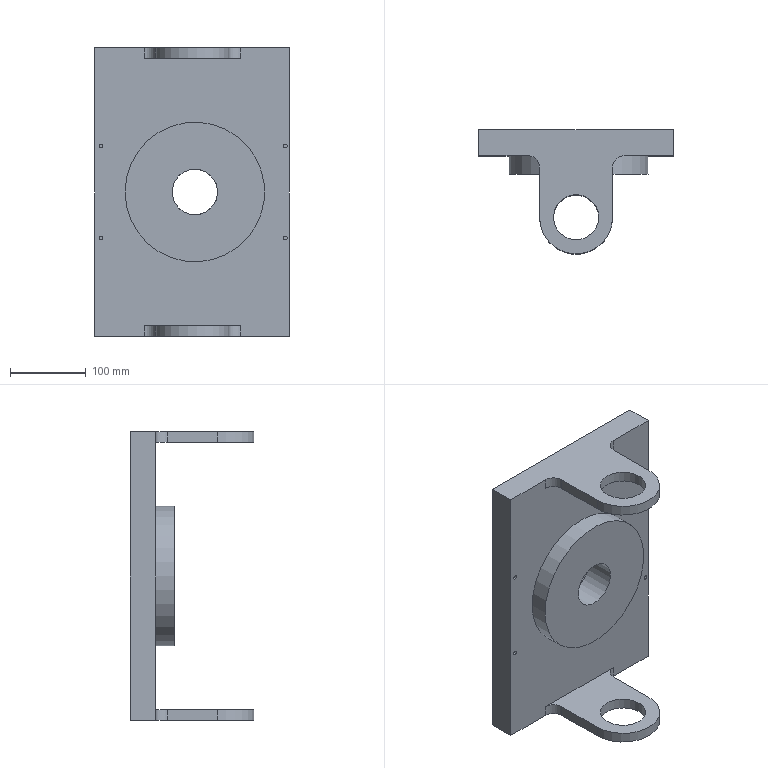Part | NX | features BREP 3 | 3 solids | 41 faces | box 256 x 163.215 x 380 mm | volume 4024571 mm3 | plane 22 | cylinder 19 | commonest cylinder face diameters 5 x4 30 x4 59.433 x2 60 x2 95 x2 96.269 x2
STEP:
#1=CARTESIAN_POINT('',(18.91,256.,-98.298));
#2=VERTEX_POINT('',#1);
#3=CARTESIAN_POINT('',(21.41,256.,-98.298));
#4=DIRECTION('',(0.,1.,0.));
#5=DIRECTION('',(-1.,0.,0.));
#6=AXIS2_PLACEMENT_3D('',#3,#4,#5);
#7=CIRCLE('',#6,2.5);
#8=EDGE_CURVE('',#2,#2,#7,.T.);
#9=ORIENTED_EDGE('',*,*,#8,.T.);
#10=EDGE_LOOP('',(#9));
#11=FACE_BOUND('',#10,.T.);
#12=CARTESIAN_POINT('',(-223.757,256.,-219.702));
#13=VERTEX_POINT('',#12);
#14=CARTESIAN_POINT('',(-221.257,256.,-219.702));
#15=DIRECTION('',(0.,1.,0.));
#16=DIRECTION('',(-1.,0.,0.));
#17=AXIS2_PLACEMENT_3D('',#14,#15,#16);
#18=CIRCLE('',#17,2.5);
#19=EDGE_CURVE('',#13,#13,#18,.T.);
#20=ORIENTED_EDGE('',*,*,#19,.T.);
#21=EDGE_LOOP('',(#20));
#22=FACE_BOUND('',#21,.T.);
#23=CARTESIAN_POINT('',(-189.579,256.,-159.));
#24=VERTEX_POINT('',#23);
#25=CARTESIAN_POINT('',(-97.711,256.,-159.));
#26=DIRECTION('',(0.,-1.,0.));
#27=DIRECTION('',(-1.,0.,0.));
#28=AXIS2_PLACEMENT_3D('',#25,#26,#27);
#29=CIRCLE('',#28,91.868);
#30=EDGE_CURVE('',#24,#24,#29,.T.);
#31=ORIENTED_EDGE('',*,*,#30,.F.);
#32=EDGE_LOOP('',(#31));
#33=FACE_BOUND('',#32,.T.);
#34=CARTESIAN_POINT('',(-38.221,256.,31.));
#35=VERTEX_POINT('',#34);
#36=CARTESIAN_POINT('',(26.51,256.,31.));
#37=VERTEX_POINT('',#36);
#38=CARTESIAN_POINT('',(26.51,256.,31.));
#39=DIRECTION('',(1.,0.,0.));
#40=VECTOR('',#39,1000.);
#41=LINE('',#38,#40);
#42=EDGE_CURVE('',#35,#37,#41,.T.);
#43=ORIENTED_EDGE('',*,*,#42,.F.);
#44=CARTESIAN_POINT('',(-38.221,256.,17.));
#45=VERTEX_POINT('',#44);
#46=CARTESIAN_POINT('',(-38.221,256.,17.));
#47=DIRECTION('',(0.,0.,-1.));
#48=VECTOR('',#47,1000.);
#49=LINE('',#46,#48);
#50=EDGE_CURVE('',#35,#45,#49,.T.);
#51=ORIENTED_EDGE('',*,*,#50,.T.);
#52=CARTESIAN_POINT('',(-164.49,256.,17.));
#53=VERTEX_POINT('',#52);
#54=CARTESIAN_POINT('',(-1006.286,256.,17.));
#55=DIRECTION('',(1.,0.,0.));
#56=VECTOR('',#55,1000.);
#57=LINE('',#54,#56);
#58=EDGE_CURVE('',#53,#45,#57,.T.);
#59=ORIENTED_EDGE('',*,*,#58,.F.);
#60=CARTESIAN_POINT('',(-164.49,256.,31.));
#61=VERTEX_POINT('',#60);
#62=CARTESIAN_POINT('',(-164.49,256.,31.));
#63=DIRECTION('',(0.,0.,1.));
#64=VECTOR('',#63,1000.);
#65=LINE('',#62,#64);
#66=EDGE_CURVE('',#53,#61,#65,.T.);
#67=ORIENTED_EDGE('',*,*,#66,.T.);
#68=CARTESIAN_POINT('',(-229.49,256.,31.));
#69=VERTEX_POINT('',#68);
#70=CARTESIAN_POINT('',(-229.49,256.,31.));
#71=DIRECTION('',(1.,0.,0.));
#72=VECTOR('',#71,1000.);
#73=LINE('',#70,#72);
#74=EDGE_CURVE('',#69,#61,#73,.T.);
#75=ORIENTED_EDGE('',*,*,#74,.F.);
#76=CARTESIAN_POINT('',(-229.49,256.,-349.));
#77=VERTEX_POINT('',#76);
#78=CARTESIAN_POINT('',(-229.49,256.,-349.));
#79=DIRECTION('',(0.,0.,1.));
#80=VECTOR('',#79,1000.);
#81=LINE('',#78,#80);
#82=EDGE_CURVE('',#77,#69,#81,.T.);
#83=ORIENTED_EDGE('',*,*,#82,.F.);
#84=CARTESIAN_POINT('',(-164.49,256.,-349.));
#85=VERTEX_POINT('',#84);
#86=CARTESIAN_POINT('',(-229.49,256.,-349.));
#87=DIRECTION('',(-1.,0.,0.));
#88=VECTOR('',#87,1000.);
#89=LINE('',#86,#88);
#90=EDGE_CURVE('',#85,#77,#89,.T.);
#91=ORIENTED_EDGE('',*,*,#90,.F.);
#92=CARTESIAN_POINT('',(-164.49,256.,-335.));
#93=VERTEX_POINT('',#92);
#94=CARTESIAN_POINT('',(-164.49,256.,-335.));
#95=DIRECTION('',(0.,0.,1.));
#96=VECTOR('',#95,1000.);
#97=LINE('',#94,#96);
#98=EDGE_CURVE('',#85,#93,#97,.T.);
#99=ORIENTED_EDGE('',*,*,#98,.T.);
#100=CARTESIAN_POINT('',(-38.221,256.,-335.));
#101=VERTEX_POINT('',#100);
#102=CARTESIAN_POINT('',(-1006.286,256.,-335.));
#103=DIRECTION('',(-1.,0.,0.));
#104=VECTOR('',#103,1000.);
#105=LINE('',#102,#104);
#106=EDGE_CURVE('',#101,#93,#105,.T.);
#107=ORIENTED_EDGE('',*,*,#106,.F.);
#108=CARTESIAN_POINT('',(-38.221,256.,-349.));
#109=VERTEX_POINT('',#108);
#110=CARTESIAN_POINT('',(-38.221,256.,-349.));
#111=DIRECTION('',(0.,0.,-1.));
#112=VECTOR('',#111,1000.);
#113=LINE('',#110,#112);
#114=EDGE_CURVE('',#101,#109,#113,.T.);
#115=ORIENTED_EDGE('',*,*,#114,.T.);
#116=CARTESIAN_POINT('',(26.51,256.,-349.));
#117=VERTEX_POINT('',#116);
#118=CARTESIAN_POINT('',(26.51,256.,-349.));
#119=DIRECTION('',(-1.,0.,0.));
#120=VECTOR('',#119,1000.);
#121=LINE('',#118,#120);
#122=EDGE_CURVE('',#117,#109,#121,.T.);
#123=ORIENTED_EDGE('',*,*,#122,.F.);
#124=CARTESIAN_POINT('',(26.51,256.,31.));
#125=DIRECTION('',(0.,0.,-1.));
#126=VECTOR('',#125,1000.);
#127=LINE('',#124,#126);
#128=EDGE_CURVE('',#37,#117,#127,.T.);
#129=ORIENTED_EDGE('',*,*,#128,.F.);
#130=EDGE_LOOP('',(#43,#51,#59,#67,#75,#83,#91,#99,#107,#115,#123,#129));
#131=FACE_BOUND('',#130,.T.);
#132=CARTESIAN_POINT('',(18.91,256.,-219.702));
#133=VERTEX_POINT('',#132);
#134=CARTESIAN_POINT('',(21.41,256.,-219.702));
#135=DIRECTION('',(0.,-1.,0.));
#136=DIRECTION('',(-1.,0.,0.));
#137=AXIS2_PLACEMENT_3D('',#134,#135,#136);
#138=CIRCLE('',#137,2.5);
#139=EDGE_CURVE('',#133,#133,#138,.T.);
#140=ORIENTED_EDGE('',*,*,#139,.F.);
#141=EDGE_LOOP('',(#140));
#142=FACE_BOUND('',#141,.T.);
#143=CARTESIAN_POINT('',(-223.757,256.,-98.298));
#144=VERTEX_POINT('',#143);
#145=CARTESIAN_POINT('',(-221.257,256.,-98.298));
#146=DIRECTION('',(0.,-1.,0.));
#147=DIRECTION('',(-1.,0.,0.));
#148=AXIS2_PLACEMENT_3D('',#145,#146,#147);
#149=CIRCLE('',#148,2.5);
#150=EDGE_CURVE('',#144,#144,#149,.T.);
#151=ORIENTED_EDGE('',*,*,#150,.F.);
#152=EDGE_LOOP('',(#151));
#153=FACE_BOUND('',#152,.T.);
#154=CARTESIAN_POINT('',(26.51,256.,31.));
#155=DIRECTION('',(0.,1.,0.));
#156=DIRECTION('',(1.,0.,0.));
#157=AXIS2_PLACEMENT_3D('',#154,#155,#156);
#158=PLANE('',#157);
#159=ADVANCED_FACE('',(#11,#22,#33,#131,#142,#153),#158,.F.);
#160=CARTESIAN_POINT('',(-97.711,232.,-189.));
#161=VERTEX_POINT('',#160);
#162=CARTESIAN_POINT('',(-97.711,232.,-159.));
#163=DIRECTION('',(0.,-1.,0.));
#164=DIRECTION('',(0.,0.,-1.));
#165=AXIS2_PLACEMENT_3D('',#162,#163,#164);
#166=CIRCLE('',#165,30.);
#167=EDGE_CURVE('',#161,#161,#166,.T.);
#168=ORIENTED_EDGE('',*,*,#167,.T.);
#169=EDGE_LOOP('',(#168));
#170=FACE_BOUND('',#169,.T.);
#171=CARTESIAN_POINT('',(-97.711,272.,-129.));
#172=VERTEX_POINT('',#171);
#173=CARTESIAN_POINT('',(-97.711,272.,-159.));
#174=DIRECTION('',(0.,-1.,0.));
#175=DIRECTION('',(0.,0.,1.));
#176=AXIS2_PLACEMENT_3D('',#173,#174,#175);
#177=CIRCLE('',#176,30.);
#178=EDGE_CURVE('',#172,#172,#177,.T.);
#179=ORIENTED_EDGE('',*,*,#178,.F.);
#180=EDGE_LOOP('',(#179));
#181=FACE_BOUND('',#180,.T.);
#182=CARTESIAN_POINT('',(-97.711,315.,-159.));
#183=DIRECTION('',(0.,-1.,0.));
#184=DIRECTION('',(-1.,0.,0.));
#185=AXIS2_PLACEMENT_3D('',#182,#183,#184);
#186=CYLINDRICAL_SURFACE('',#185,30.);
#187=ADVANCED_FACE('',(#170,#181),#186,.F.);
#188=ORIENTED_EDGE('',*,*,#122,.T.);
#189=CARTESIAN_POINT('',(-53.221,241.,-349.));
#190=VERTEX_POINT('',#189);
#191=CARTESIAN_POINT('',(-38.221,241.,-349.));
#192=DIRECTION('',(0.,0.,1.));
#193=DIRECTION('',(0.,-1.,0.));
#194=AXIS2_PLACEMENT_3D('',#191,#192,#193);
#195=CIRCLE('',#194,15.);
#196=EDGE_CURVE('',#109,#190,#195,.T.);
#197=ORIENTED_EDGE('',*,*,#196,.T.);
#198=CARTESIAN_POINT('',(-53.221,174.92,-349.));
#199=VERTEX_POINT('',#198);
#200=CARTESIAN_POINT('',(-53.221,290.,-349.));
#201=DIRECTION('',(0.,1.,0.));
#202=VECTOR('',#201,1000.);
#203=LINE('',#200,#202);
#204=EDGE_CURVE('',#199,#190,#203,.T.);
#205=ORIENTED_EDGE('',*,*,#204,.F.);
#206=CARTESIAN_POINT('',(-149.49,174.92,-349.));
#207=VERTEX_POINT('',#206);
#208=CARTESIAN_POINT('',(-101.355,174.92,-349.));
#209=DIRECTION('',(0.,0.,1.));
#210=DIRECTION('',(-1.,0.,0.));
#211=AXIS2_PLACEMENT_3D('',#208,#209,#210);
#212=CIRCLE('',#211,48.135);
#213=EDGE_CURVE('',#207,#199,#212,.T.);
#214=ORIENTED_EDGE('',*,*,#213,.F.);
#215=CARTESIAN_POINT('',(-149.49,241.,-349.));
#216=VERTEX_POINT('',#215);
#217=CARTESIAN_POINT('',(-149.49,174.92,-349.));
#218=DIRECTION('',(0.,-1.,0.));
#219=VECTOR('',#218,1000.);
#220=LINE('',#217,#219);
#221=EDGE_CURVE('',#216,#207,#220,.T.);
#222=ORIENTED_EDGE('',*,*,#221,.F.);
#223=CARTESIAN_POINT('',(-164.49,241.,-349.));
#224=DIRECTION('',(0.,0.,1.));
#225=DIRECTION('',(0.,-1.,0.));
#226=AXIS2_PLACEMENT_3D('',#223,#224,#225);
#227=CIRCLE('',#226,15.);
#228=EDGE_CURVE('',#216,#85,#227,.T.);
#229=ORIENTED_EDGE('',*,*,#228,.T.);
#230=ORIENTED_EDGE('',*,*,#90,.T.);
#231=CARTESIAN_POINT('',(-229.49,290.,-349.));
#232=VERTEX_POINT('',#231);
#233=CARTESIAN_POINT('',(-229.49,290.,-349.));
#234=DIRECTION('',(0.,-1.,0.));
#235=VECTOR('',#234,1000.);
#236=LINE('',#233,#235);
#237=EDGE_CURVE('',#232,#77,#236,.T.);
#238=ORIENTED_EDGE('',*,*,#237,.F.);
#239=CARTESIAN_POINT('',(26.51,290.,-349.));
#240=VERTEX_POINT('',#239);
#241=CARTESIAN_POINT('',(26.51,290.,-349.));
#242=DIRECTION('',(-1.,0.,0.));
#243=VECTOR('',#242,1000.);
#244=LINE('',#241,#243);
#245=EDGE_CURVE('',#240,#232,#244,.T.);
#246=ORIENTED_EDGE('',*,*,#245,.F.);
#247=CARTESIAN_POINT('',(26.51,256.,-349.));
#248=DIRECTION('',(0.,1.,0.));
#249=VECTOR('',#248,1000.);
#250=LINE('',#247,#249);
#251=EDGE_CURVE('',#117,#240,#250,.T.);
#252=ORIENTED_EDGE('',*,*,#251,.F.);
#253=EDGE_LOOP('',(#188,#197,#205,#214,#222,#229,#230,#238,#246,#252));
#254=FACE_BOUND('',#253,.T.);
#255=CARTESIAN_POINT('',(-131.072,174.92,-349.));
#256=VERTEX_POINT('',#255);
#257=CARTESIAN_POINT('',(-101.355,174.92,-349.));
#258=DIRECTION('',(0.,0.,1.));
#259=DIRECTION('',(-1.,0.,0.));
#260=AXIS2_PLACEMENT_3D('',#257,#258,#259);
#261=CIRCLE('',#260,29.717);
#262=EDGE_CURVE('',#256,#256,#261,.T.);
#263=ORIENTED_EDGE('',*,*,#262,.T.);
#264=EDGE_LOOP('',(#263));
#265=FACE_BOUND('',#264,.T.);
#266=CARTESIAN_POINT('',(26.51,256.,-349.));
#267=DIRECTION('',(0.,0.,1.));
#268=DIRECTION('',(0.,1.,0.));
#269=AXIS2_PLACEMENT_3D('',#266,#267,#268);
#270=PLANE('',#269);
#271=ADVANCED_FACE('',(#254,#265),#270,.F.);
#272=CARTESIAN_POINT('',(-32.711,290.,-159.));
#273=VERTEX_POINT('',#272);
#274=CARTESIAN_POINT('',(-97.711,290.,-159.));
#275=DIRECTION('',(0.,-1.,0.));
#276=DIRECTION('',(1.,0.,0.));
#277=AXIS2_PLACEMENT_3D('',#274,#275,#276);
#278=CIRCLE('',#277,65.);
#279=EDGE_CURVE('',#273,#273,#278,.T.);
#280=ORIENTED_EDGE('',*,*,#279,.T.);
#281=EDGE_LOOP('',(#280));
#282=FACE_BOUND('',#281,.T.);
#283=ORIENTED_EDGE('',*,*,#245,.T.);
#284=CARTESIAN_POINT('',(-229.49,290.,31.));
#285=VERTEX_POINT('',#284);
#286=CARTESIAN_POINT('',(-229.49,290.,31.));
#287=DIRECTION('',(0.,0.,-1.));
#288=VECTOR('',#287,1000.);
#289=LINE('',#286,#288);
#290=EDGE_CURVE('',#285,#232,#289,.T.);
#291=ORIENTED_EDGE('',*,*,#290,.F.);
#292=CARTESIAN_POINT('',(26.51,290.,31.));
#293=VERTEX_POINT('',#292);
#294=CARTESIAN_POINT('',(26.51,290.,31.));
#295=DIRECTION('',(1.,0.,0.));
#296=VECTOR('',#295,1000.);
#297=LINE('',#294,#296);
#298=EDGE_CURVE('',#285,#293,#297,.T.);
#299=ORIENTED_EDGE('',*,*,#298,.T.);
#300=CARTESIAN_POINT('',(26.51,290.,-349.));
#301=DIRECTION('',(0.,0.,1.));
#302=VECTOR('',#301,1000.);
#303=LINE('',#300,#302);
#304=EDGE_CURVE('',#240,#293,#303,.T.);
#305=ORIENTED_EDGE('',*,*,#304,.F.);
#306=EDGE_LOOP('',(#283,#291,#299,#305));
#307=FACE_BOUND('',#306,.T.);
#308=CARTESIAN_POINT('',(26.51,290.,-349.));
#309=DIRECTION('',(0.,-1.,0.));
#310=DIRECTION('',(-1.,0.,0.));
#311=AXIS2_PLACEMENT_3D('',#308,#309,#310);
#312=PLANE('',#311);
#313=ADVANCED_FACE('',(#282,#307),#312,.F.);
#314=ORIENTED_EDGE('',*,*,#298,.F.);
#315=CARTESIAN_POINT('',(-229.49,256.,31.));
#316=DIRECTION('',(0.,1.,0.));
#317=VECTOR('',#316,1000.);
#318=LINE('',#315,#317);
#319=EDGE_CURVE('',#69,#285,#318,.T.);
#320=ORIENTED_EDGE('',*,*,#319,.F.);
#321=ORIENTED_EDGE('',*,*,#74,.T.);
#322=CARTESIAN_POINT('',(-149.49,241.,31.));
#323=VERTEX_POINT('',#322);
#324=CARTESIAN_POINT('',(-164.49,241.,31.));
#325=DIRECTION('',(0.,0.,-1.));
#326=DIRECTION('',(-1.,0.,0.));
#327=AXIS2_PLACEMENT_3D('',#324,#325,#326);
#328=CIRCLE('',#327,15.);
#329=EDGE_CURVE('',#61,#323,#328,.T.);
#330=ORIENTED_EDGE('',*,*,#329,.T.);
#331=CARTESIAN_POINT('',(-149.49,174.92,31.));
#332=VERTEX_POINT('',#331);
#333=CARTESIAN_POINT('',(-149.49,174.92,31.));
#334=DIRECTION('',(0.,1.,0.));
#335=VECTOR('',#334,1000.);
#336=LINE('',#333,#335);
#337=EDGE_CURVE('',#332,#323,#336,.T.);
#338=ORIENTED_EDGE('',*,*,#337,.F.);
#339=CARTESIAN_POINT('',(-53.221,174.92,31.));
#340=VERTEX_POINT('',#339);
#341=CARTESIAN_POINT('',(-101.355,174.92,31.));
#342=DIRECTION('',(0.,0.,-1.));
#343=DIRECTION('',(-1.,0.,0.));
#344=AXIS2_PLACEMENT_3D('',#341,#342,#343);
#345=CIRCLE('',#344,48.135);
#346=EDGE_CURVE('',#340,#332,#345,.T.);
#347=ORIENTED_EDGE('',*,*,#346,.F.);
#348=CARTESIAN_POINT('',(-53.221,241.,31.));
#349=VERTEX_POINT('',#348);
#350=CARTESIAN_POINT('',(-53.221,290.,31.));
#351=DIRECTION('',(0.,-1.,0.));
#352=VECTOR('',#351,1000.);
#353=LINE('',#350,#352);
#354=EDGE_CURVE('',#349,#340,#353,.T.);
#355=ORIENTED_EDGE('',*,*,#354,.F.);
#356=CARTESIAN_POINT('',(-38.221,241.,31.));
#357=DIRECTION('',(0.,0.,-1.));
#358=DIRECTION('',(-1.,0.,0.));
#359=AXIS2_PLACEMENT_3D('',#356,#357,#358);
#360=CIRCLE('',#359,15.);
#361=EDGE_CURVE('',#349,#35,#360,.T.);
#362=ORIENTED_EDGE('',*,*,#361,.T.);
#363=ORIENTED_EDGE('',*,*,#42,.T.);
#364=CARTESIAN_POINT('',(26.51,290.,31.));
#365=DIRECTION('',(0.,-1.,0.));
#366=VECTOR('',#365,1000.);
#367=LINE('',#364,#366);
#368=EDGE_CURVE('',#293,#37,#367,.T.);
#369=ORIENTED_EDGE('',*,*,#368,.F.);
#370=EDGE_LOOP('',(#314,#320,#321,#330,#338,#347,#355,#362,#363,#369));
#371=FACE_BOUND('',#370,.T.);
#372=CARTESIAN_POINT('',(-131.072,174.92,31.));
#373=VERTEX_POINT('',#372);
#374=CARTESIAN_POINT('',(-101.355,174.92,31.));
#375=DIRECTION('',(0.,0.,-1.));
#376=DIRECTION('',(-1.,0.,0.));
#377=AXIS2_PLACEMENT_3D('',#374,#375,#376);
#378=CIRCLE('',#377,29.717);
#379=EDGE_CURVE('',#373,#373,#378,.T.);
#380=ORIENTED_EDGE('',*,*,#379,.T.);
#381=EDGE_LOOP('',(#380));
#382=FACE_BOUND('',#381,.T.);
#383=CARTESIAN_POINT('',(26.51,290.,31.));
#384=DIRECTION('',(0.,0.,-1.));
#385=DIRECTION('',(1.,0.,0.));
#386=AXIS2_PLACEMENT_3D('',#383,#384,#385);
#387=PLANE('',#386);
#388=ADVANCED_FACE('',(#371,#382),#387,.F.);
#389=ORIENTED_EDGE('',*,*,#251,.T.);
#390=ORIENTED_EDGE('',*,*,#304,.T.);
#391=ORIENTED_EDGE('',*,*,#368,.T.);
#392=ORIENTED_EDGE('',*,*,#128,.T.);
#393=EDGE_LOOP('',(#389,#390,#391,#392));
#394=FACE_BOUND('',#393,.T.);
#395=CARTESIAN_POINT('',(26.51,0.,0.));
#396=DIRECTION('',(1.,0.,0.));
#397=DIRECTION('',(0.,0.,1.));
#398=AXIS2_PLACEMENT_3D('',#395,#396,#397);
#399=PLANE('',#398);
#400=ADVANCED_FACE('',(#394),#399,.T.);
#401=ORIENTED_EDGE('',*,*,#204,.T.);
#402=CARTESIAN_POINT('',(-53.221,241.,-335.));
#403=VERTEX_POINT('',#402);
#404=CARTESIAN_POINT('',(-53.221,241.,-335.));
#405=DIRECTION('',(0.,0.,1.));
#406=VECTOR('',#405,1000.);
#407=LINE('',#404,#406);
#408=EDGE_CURVE('',#190,#403,#407,.T.);
#409=ORIENTED_EDGE('',*,*,#408,.T.);
#410=CARTESIAN_POINT('',(-53.221,174.92,-335.));
#411=VERTEX_POINT('',#410);
#412=CARTESIAN_POINT('',(-53.221,290.,-335.));
#413=DIRECTION('',(0.,1.,0.));
#414=VECTOR('',#413,1000.);
#415=LINE('',#412,#414);
#416=EDGE_CURVE('',#411,#403,#415,.T.);
#417=ORIENTED_EDGE('',*,*,#416,.F.);
#418=CARTESIAN_POINT('',(-53.221,174.92,-335.));
#419=DIRECTION('',(0.,0.,1.));
#420=VECTOR('',#419,1000.);
#421=LINE('',#418,#420);
#422=EDGE_CURVE('',#199,#411,#421,.T.);
#423=ORIENTED_EDGE('',*,*,#422,.F.);
#424=EDGE_LOOP('',(#401,#409,#417,#423));
#425=FACE_BOUND('',#424,.T.);
#426=CARTESIAN_POINT('',(-53.221,290.,-335.));
#427=DIRECTION('',(-1.,0.,0.));
#428=DIRECTION('',(0.,0.,1.));
#429=AXIS2_PLACEMENT_3D('',#426,#427,#428);
#430=PLANE('',#429);
#431=ADVANCED_FACE('',(#425),#430,.F.);
#432=CARTESIAN_POINT('',(-53.221,241.,17.));
#433=VERTEX_POINT('',#432);
#434=CARTESIAN_POINT('',(-53.221,174.92,17.));
#435=VERTEX_POINT('',#434);
#436=CARTESIAN_POINT('',(-53.221,290.,17.));
#437=DIRECTION('',(0.,-1.,0.));
#438=VECTOR('',#437,1000.);
#439=LINE('',#436,#438);
#440=EDGE_CURVE('',#433,#435,#439,.T.);
#441=ORIENTED_EDGE('',*,*,#440,.F.);
#442=CARTESIAN_POINT('',(-53.221,241.,31.));
#443=DIRECTION('',(0.,0.,1.));
#444=VECTOR('',#443,1000.);
#445=LINE('',#442,#444);
#446=EDGE_CURVE('',#433,#349,#445,.T.);
#447=ORIENTED_EDGE('',*,*,#446,.T.);
#448=ORIENTED_EDGE('',*,*,#354,.T.);
#449=CARTESIAN_POINT('',(-53.221,174.92,17.));
#450=DIRECTION('',(0.,0.,1.));
#451=VECTOR('',#450,1000.);
#452=LINE('',#449,#451);
#453=EDGE_CURVE('',#435,#340,#452,.T.);
#454=ORIENTED_EDGE('',*,*,#453,.F.);
#455=EDGE_LOOP('',(#441,#447,#448,#454));
#456=FACE_BOUND('',#455,.T.);
#457=CARTESIAN_POINT('',(-53.221,290.,-335.));
#458=DIRECTION('',(-1.,0.,0.));
#459=DIRECTION('',(0.,0.,1.));
#460=AXIS2_PLACEMENT_3D('',#457,#458,#459);
#461=PLANE('',#460);
#462=ADVANCED_FACE('',(#456),#461,.F.);
#463=CARTESIAN_POINT('',(-149.49,241.,-335.));
#464=VERTEX_POINT('',#463);
#465=CARTESIAN_POINT('',(-149.49,174.92,-335.));
#466=VERTEX_POINT('',#465);
#467=CARTESIAN_POINT('',(-149.49,174.92,-335.));
#468=DIRECTION('',(0.,-1.,0.));
#469=VECTOR('',#468,1000.);
#470=LINE('',#467,#469);
#471=EDGE_CURVE('',#464,#466,#470,.T.);
#472=ORIENTED_EDGE('',*,*,#471,.F.);
#473=CARTESIAN_POINT('',(-149.49,241.,-349.));
#474=DIRECTION('',(0.,0.,-1.));
#475=VECTOR('',#474,1000.);
#476=LINE('',#473,#475);
#477=EDGE_CURVE('',#464,#216,#476,.T.);
#478=ORIENTED_EDGE('',*,*,#477,.T.);
#479=ORIENTED_EDGE('',*,*,#221,.T.);
#480=CARTESIAN_POINT('',(-149.49,174.92,-335.));
#481=DIRECTION('',(0.,0.,1.));
#482=VECTOR('',#481,1000.);
#483=LINE('',#480,#482);
#484=EDGE_CURVE('',#207,#466,#483,.T.);
#485=ORIENTED_EDGE('',*,*,#484,.T.);
#486=EDGE_LOOP('',(#472,#478,#479,#485));
#487=FACE_BOUND('',#486,.T.);
#488=CARTESIAN_POINT('',(-149.49,174.92,-335.));
#489=DIRECTION('',(1.,0.,0.));
#490=DIRECTION('',(0.,-1.,0.));
#491=AXIS2_PLACEMENT_3D('',#488,#489,#490);
#492=PLANE('',#491);
#493=ADVANCED_FACE('',(#487),#492,.F.);
#494=ORIENTED_EDGE('',*,*,#337,.T.);
#495=CARTESIAN_POINT('',(-149.49,241.,17.));
#496=VERTEX_POINT('',#495);
#497=CARTESIAN_POINT('',(-149.49,241.,17.));
#498=DIRECTION('',(0.,0.,-1.));
#499=VECTOR('',#498,1000.);
#500=LINE('',#497,#499);
#501=EDGE_CURVE('',#323,#496,#500,.T.);
#502=ORIENTED_EDGE('',*,*,#501,.T.);
#503=CARTESIAN_POINT('',(-149.49,174.92,17.));
#504=VERTEX_POINT('',#503);
#505=CARTESIAN_POINT('',(-149.49,174.92,17.));
#506=DIRECTION('',(0.,1.,0.));
#507=VECTOR('',#506,1000.);
#508=LINE('',#505,#507);
#509=EDGE_CURVE('',#504,#496,#508,.T.);
#510=ORIENTED_EDGE('',*,*,#509,.F.);
#511=CARTESIAN_POINT('',(-149.49,174.92,17.));
#512=DIRECTION('',(0.,0.,1.));
#513=VECTOR('',#512,1000.);
#514=LINE('',#511,#513);
#515=EDGE_CURVE('',#504,#332,#514,.T.);
#516=ORIENTED_EDGE('',*,*,#515,.T.);
#517=EDGE_LOOP('',(#494,#502,#510,#516));
#518=FACE_BOUND('',#517,.T.);
#519=CARTESIAN_POINT('',(-149.49,174.92,-335.));
#520=DIRECTION('',(1.,0.,0.));
#521=DIRECTION('',(0.,-1.,0.));
#522=AXIS2_PLACEMENT_3D('',#519,#520,#521);
#523=PLANE('',#522);
#524=ADVANCED_FACE('',(#518),#523,.F.);
#525=ORIENTED_EDGE('',*,*,#346,.T.);
#526=ORIENTED_EDGE('',*,*,#515,.F.);
#527=CARTESIAN_POINT('',(-101.355,174.92,17.));
#528=DIRECTION('',(0.,0.,-1.));
#529=DIRECTION('',(-1.,0.,0.));
#530=AXIS2_PLACEMENT_3D('',#527,#528,#529);
#531=CIRCLE('',#530,48.135);
#532=EDGE_CURVE('',#435,#504,#531,.T.);
#533=ORIENTED_EDGE('',*,*,#532,.F.);
#534=ORIENTED_EDGE('',*,*,#453,.T.);
#535=EDGE_LOOP('',(#525,#526,#533,#534));
#536=FACE_BOUND('',#535,.T.);
#537=CARTESIAN_POINT('',(-101.355,174.92,17.));
#538=DIRECTION('',(0.,0.,1.));
#539=DIRECTION('',(-1.,0.,0.));
#540=AXIS2_PLACEMENT_3D('',#537,#538,#539);
#541=CYLINDRICAL_SURFACE('',#540,48.135);
#542=ADVANCED_FACE('',(#536),#541,.T.);
#543=CARTESIAN_POINT('',(-131.072,174.92,17.));
#544=VERTEX_POINT('',#543);
#545=CARTESIAN_POINT('',(-101.355,174.92,17.));
#546=DIRECTION('',(0.,0.,-1.));
#547=DIRECTION('',(-1.,0.,0.));
#548=AXIS2_PLACEMENT_3D('',#545,#546,#547);
#549=CIRCLE('',#548,29.717);
#550=EDGE_CURVE('',#544,#544,#549,.T.);
#551=ORIENTED_EDGE('',*,*,#550,.T.);
#552=EDGE_LOOP('',(#551));
#553=FACE_BOUND('',#552,.T.);
#554=ORIENTED_EDGE('',*,*,#379,.F.);
#555=EDGE_LOOP('',(#554));
#556=FACE_BOUND('',#555,.T.);
#557=CARTESIAN_POINT('',(-101.355,174.92,17.));
#558=DIRECTION('',(0.,0.,1.));
#559=DIRECTION('',(-1.,0.,0.));
#560=AXIS2_PLACEMENT_3D('',#557,#558,#559);
#561=CYLINDRICAL_SURFACE('',#560,29.717);
#562=ADVANCED_FACE('',(#553,#556),#561,.F.);
#563=ORIENTED_EDGE('',*,*,#509,.T.);
#564=CARTESIAN_POINT('',(-164.49,241.,17.));
#565=DIRECTION('',(0.,0.,1.));
#566=DIRECTION('',(-1.,0.,0.));
#567=AXIS2_PLACEMENT_3D('',#564,#565,#566);
#568=CIRCLE('',#567,15.);
#569=EDGE_CURVE('',#496,#53,#568,.T.);
#570=ORIENTED_EDGE('',*,*,#569,.T.);
#571=ORIENTED_EDGE('',*,*,#58,.T.);
#572=CARTESIAN_POINT('',(-38.221,241.,17.));
#573=DIRECTION('',(0.,0.,1.));
#574=DIRECTION('',(-1.,0.,0.));
#575=AXIS2_PLACEMENT_3D('',#572,#573,#574);
#576=CIRCLE('',#575,15.);
#577=EDGE_CURVE('',#45,#433,#576,.T.);
#578=ORIENTED_EDGE('',*,*,#577,.T.);
#579=ORIENTED_EDGE('',*,*,#440,.T.);
#580=ORIENTED_EDGE('',*,*,#532,.T.);
#581=EDGE_LOOP('',(#563,#570,#571,#578,#579,#580));
#582=FACE_BOUND('',#581,.T.);
#583=ORIENTED_EDGE('',*,*,#550,.F.);
#584=EDGE_LOOP('',(#583));
#585=FACE_BOUND('',#584,.T.);
#586=CARTESIAN_POINT('',(-101.355,174.92,17.));
#587=DIRECTION('',(0.,0.,-1.));
#588=DIRECTION('',(1.,0.,0.));
#589=AXIS2_PLACEMENT_3D('',#586,#587,#588);
#590=PLANE('',#589);
#591=ADVANCED_FACE('',(#582,#585),#590,.T.);
#592=ORIENTED_EDGE('',*,*,#213,.T.);
#593=ORIENTED_EDGE('',*,*,#422,.T.);
#594=CARTESIAN_POINT('',(-101.355,174.92,-335.));
#595=DIRECTION('',(0.,0.,1.));
#596=DIRECTION('',(-1.,0.,0.));
#597=AXIS2_PLACEMENT_3D('',#594,#595,#596);
#598=CIRCLE('',#597,48.135);
#599=EDGE_CURVE('',#466,#411,#598,.T.);
#600=ORIENTED_EDGE('',*,*,#599,.F.);
#601=ORIENTED_EDGE('',*,*,#484,.F.);
#602=EDGE_LOOP('',(#592,#593,#600,#601));
#603=FACE_BOUND('',#602,.T.);
#604=CARTESIAN_POINT('',(-101.355,174.92,-335.));
#605=DIRECTION('',(0.,0.,-1.));
#606=DIRECTION('',(-1.,0.,0.));
#607=AXIS2_PLACEMENT_3D('',#604,#605,#606);
#608=CYLINDRICAL_SURFACE('',#607,48.135);
#609=ADVANCED_FACE('',(#603),#608,.T.);
#610=CARTESIAN_POINT('',(-131.072,174.92,-335.));
#611=VERTEX_POINT('',#610);
#612=CARTESIAN_POINT('',(-101.355,174.92,-335.));
#613=DIRECTION('',(0.,0.,1.));
#614=DIRECTION('',(-1.,0.,0.));
#615=AXIS2_PLACEMENT_3D('',#612,#613,#614);
#616=CIRCLE('',#615,29.717);
#617=EDGE_CURVE('',#611,#611,#616,.T.);
#618=ORIENTED_EDGE('',*,*,#617,.T.);
#619=EDGE_LOOP('',(#618));
#620=FACE_BOUND('',#619,.T.);
#621=ORIENTED_EDGE('',*,*,#262,.F.);
#622=EDGE_LOOP('',(#621));
#623=FACE_BOUND('',#622,.T.);
#624=CARTESIAN_POINT('',(-101.355,174.92,-335.));
#625=DIRECTION('',(0.,0.,-1.));
#626=DIRECTION('',(-1.,0.,0.));
#627=AXIS2_PLACEMENT_3D('',#624,#625,#626);
#628=CYLINDRICAL_SURFACE('',#627,29.717);
#629=ADVANCED_FACE('',(#620,#623),#628,.F.);
#630=ORIENTED_EDGE('',*,*,#416,.T.);
#631=CARTESIAN_POINT('',(-38.221,241.,-335.));
#632=DIRECTION('',(0.,0.,-1.));
#633=DIRECTION('',(0.,-1.,0.));
#634=AXIS2_PLACEMENT_3D('',#631,#632,#633);
#635=CIRCLE('',#634,15.);
#636=EDGE_CURVE('',#403,#101,#635,.T.);
#637=ORIENTED_EDGE('',*,*,#636,.T.);
#638=ORIENTED_EDGE('',*,*,#106,.T.);
#639=CARTESIAN_POINT('',(-164.49,241.,-335.));
#640=DIRECTION('',(0.,0.,-1.));
#641=DIRECTION('',(0.,-1.,0.));
#642=AXIS2_PLACEMENT_3D('',#639,#640,#641);
#643=CIRCLE('',#642,15.);
#644=EDGE_CURVE('',#93,#464,#643,.T.);
#645=ORIENTED_EDGE('',*,*,#644,.T.);
#646=ORIENTED_EDGE('',*,*,#471,.T.);
#647=ORIENTED_EDGE('',*,*,#599,.T.);
#648=EDGE_LOOP('',(#630,#637,#638,#645,#646,#647));
#649=FACE_BOUND('',#648,.T.);
#650=ORIENTED_EDGE('',*,*,#617,.F.);
#651=EDGE_LOOP('',(#650));
#652=FACE_BOUND('',#651,.T.);
#653=CARTESIAN_POINT('',(-101.355,174.92,-335.));
#654=DIRECTION('',(0.,0.,1.));
#655=DIRECTION('',(1.,0.,0.));
#656=AXIS2_PLACEMENT_3D('',#653,#654,#655);
#657=PLANE('',#656);
#658=ADVANCED_FACE('',(#649,#652),#657,.T.);
#659=ORIENTED_EDGE('',*,*,#82,.T.);
#660=ORIENTED_EDGE('',*,*,#319,.T.);
#661=ORIENTED_EDGE('',*,*,#290,.T.);
#662=ORIENTED_EDGE('',*,*,#237,.T.);
#663=EDGE_LOOP('',(#659,#660,#661,#662));
#664=FACE_BOUND('',#663,.T.);
#665=CARTESIAN_POINT('',(-229.49,0.,0.));
#666=DIRECTION('',(-1.,0.,0.));
#667=DIRECTION('',(0.,0.,-1.));
#668=AXIS2_PLACEMENT_3D('',#665,#666,#667);
#669=PLANE('',#668);
#670=ADVANCED_FACE('',(#664),#669,.T.);
#671=ORIENTED_EDGE('',*,*,#577,.F.);
#672=ORIENTED_EDGE('',*,*,#50,.F.);
#673=ORIENTED_EDGE('',*,*,#361,.F.);
#674=ORIENTED_EDGE('',*,*,#446,.F.);
#675=EDGE_LOOP('',(#671,#672,#673,#674));
#676=FACE_BOUND('',#675,.T.);
#677=CARTESIAN_POINT('',(-38.221,241.,-335.));
#678=DIRECTION('',(0.,0.,-1.));
#679=DIRECTION('',(1.,0.,0.));
#680=AXIS2_PLACEMENT_3D('',#677,#678,#679);
#681=CYLINDRICAL_SURFACE('',#680,15.);
#682=ADVANCED_FACE('',(#676),#681,.F.);
#683=ORIENTED_EDGE('',*,*,#329,.F.);
#684=ORIENTED_EDGE('',*,*,#66,.F.);
#685=ORIENTED_EDGE('',*,*,#569,.F.);
#686=ORIENTED_EDGE('',*,*,#501,.F.);
#687=EDGE_LOOP('',(#683,#684,#685,#686));
#688=FACE_BOUND('',#687,.T.);
#689=CARTESIAN_POINT('',(-164.49,241.,-335.));
#690=DIRECTION('',(0.,0.,1.));
#691=DIRECTION('',(-1.,0.,0.));
#692=AXIS2_PLACEMENT_3D('',#689,#690,#691);
#693=CYLINDRICAL_SURFACE('',#692,15.);
#694=ADVANCED_FACE('',(#688),#693,.F.);
#695=ORIENTED_EDGE('',*,*,#644,.F.);
#696=ORIENTED_EDGE('',*,*,#98,.F.);
#697=ORIENTED_EDGE('',*,*,#228,.F.);
#698=ORIENTED_EDGE('',*,*,#477,.F.);
#699=EDGE_LOOP('',(#695,#696,#697,#698));
#700=FACE_BOUND('',#699,.T.);
#701=CARTESIAN_POINT('',(-164.49,241.,-335.));
#702=DIRECTION('',(0.,0.,1.));
#703=DIRECTION('',(-1.,0.,0.));
#704=AXIS2_PLACEMENT_3D('',#701,#702,#703);
#705=CYLINDRICAL_SURFACE('',#704,15.);
#706=ADVANCED_FACE('',(#700),#705,.F.);
#707=ORIENTED_EDGE('',*,*,#196,.F.);
#708=ORIENTED_EDGE('',*,*,#114,.F.);
#709=ORIENTED_EDGE('',*,*,#636,.F.);
#710=ORIENTED_EDGE('',*,*,#408,.F.);
#711=EDGE_LOOP('',(#707,#708,#709,#710));
#712=FACE_BOUND('',#711,.T.);
#713=CARTESIAN_POINT('',(-38.221,241.,-335.));
#714=DIRECTION('',(0.,0.,-1.));
#715=DIRECTION('',(1.,0.,0.));
#716=AXIS2_PLACEMENT_3D('',#713,#714,#715);
#717=CYLINDRICAL_SURFACE('',#716,15.);
#718=ADVANCED_FACE('',(#712),#717,.F.);
#719=CARTESIAN_POINT('',(-189.579,232.,-159.));
#720=VERTEX_POINT('',#719);
#721=CARTESIAN_POINT('',(-97.711,232.,-159.));
#722=DIRECTION('',(0.,-1.,0.));
#723=DIRECTION('',(-1.,0.,0.));
#724=AXIS2_PLACEMENT_3D('',#721,#722,#723);
#725=CIRCLE('',#724,91.868);
#726=EDGE_CURVE('',#720,#720,#725,.T.);
#727=ORIENTED_EDGE('',*,*,#726,.F.);
#728=EDGE_LOOP('',(#727));
#729=FACE_BOUND('',#728,.T.);
#730=ORIENTED_EDGE('',*,*,#30,.T.);
#731=EDGE_LOOP('',(#730));
#732=FACE_BOUND('',#731,.T.);
#733=CARTESIAN_POINT('',(-97.711,259.,-159.));
#734=DIRECTION('',(0.,-1.,0.));
#735=DIRECTION('',(-1.,0.,0.));
#736=AXIS2_PLACEMENT_3D('',#733,#734,#735);
#737=CYLINDRICAL_SURFACE('',#736,91.868);
#738=ADVANCED_FACE('',(#729,#732),#737,.T.);
#739=ORIENTED_EDGE('',*,*,#167,.F.);
#740=EDGE_LOOP('',(#739));
#741=FACE_BOUND('',#740,.T.);
#742=ORIENTED_EDGE('',*,*,#726,.T.);
#743=EDGE_LOOP('',(#742));
#744=FACE_BOUND('',#743,.T.);
#745=CARTESIAN_POINT('',(-97.711,232.,-159.));
#746=DIRECTION('',(0.,-1.,0.));
#747=DIRECTION('',(0.,0.,1.));
#748=AXIS2_PLACEMENT_3D('',#745,#746,#747);
#749=PLANE('',#748);
#750=ADVANCED_FACE('',(#741,#744),#749,.T.);
#751=CARTESIAN_POINT('',(-97.711,272.,-94.));
#752=VERTEX_POINT('',#751);
#753=CARTESIAN_POINT('',(-97.711,272.,-159.));
#754=DIRECTION('',(0.,-1.,0.));
#755=DIRECTION('',(0.,0.,1.));
#756=AXIS2_PLACEMENT_3D('',#753,#754,#755);
#757=CIRCLE('',#756,65.);
#758=EDGE_CURVE('',#752,#752,#757,.T.);
#759=ORIENTED_EDGE('',*,*,#758,.T.);
#760=EDGE_LOOP('',(#759));
#761=FACE_BOUND('',#760,.T.);
#762=ORIENTED_EDGE('',*,*,#279,.F.);
#763=EDGE_LOOP('',(#762));
#764=FACE_BOUND('',#763,.T.);
#765=CARTESIAN_POINT('',(-97.711,272.,-159.));
#766=DIRECTION('',(0.,1.,0.));
#767=DIRECTION('',(0.,0.,-1.));
#768=AXIS2_PLACEMENT_3D('',#765,#766,#767);
#769=CYLINDRICAL_SURFACE('',#768,65.);
#770=ADVANCED_FACE('',(#761,#764),#769,.F.);
#771=ORIENTED_EDGE('',*,*,#758,.F.);
#772=EDGE_LOOP('',(#771));
#773=FACE_BOUND('',#772,.T.);
#774=ORIENTED_EDGE('',*,*,#178,.T.);
#775=EDGE_LOOP('',(#774));
#776=FACE_BOUND('',#775,.T.);
#777=CARTESIAN_POINT('',(-97.711,272.,-159.));
#778=DIRECTION('',(0.,1.,0.));
#779=DIRECTION('',(0.,0.,-1.));
#780=AXIS2_PLACEMENT_3D('',#777,#778,#779);
#781=PLANE('',#780);
#782=ADVANCED_FACE('',(#773,#776),#781,.T.);
#783=CARTESIAN_POINT('',(-223.757,266.,-219.702));
#784=VERTEX_POINT('',#783);
#785=CARTESIAN_POINT('',(-221.257,266.,-219.702));
#786=DIRECTION('',(0.,1.,0.));
#787=DIRECTION('',(-1.,0.,0.));
#788=AXIS2_PLACEMENT_3D('',#785,#786,#787);
#789=CIRCLE('',#788,2.5);
#790=EDGE_CURVE('',#784,#784,#789,.T.);
#791=ORIENTED_EDGE('',*,*,#790,.T.);
#792=EDGE_LOOP('',(#791));
#793=FACE_BOUND('',#792,.T.);
#794=ORIENTED_EDGE('',*,*,#19,.F.);
#795=EDGE_LOOP('',(#794));
#796=FACE_BOUND('',#795,.T.);
#797=CARTESIAN_POINT('',(-221.257,266.,-219.702));
#798=DIRECTION('',(0.,-1.,0.));
#799=DIRECTION('',(-1.,0.,0.));
#800=AXIS2_PLACEMENT_3D('',#797,#798,#799);
#801=CYLINDRICAL_SURFACE('',#800,2.5);
#802=ADVANCED_FACE('',(#793,#796),#801,.F.);
#803=ORIENTED_EDGE('',*,*,#790,.F.);
#804=EDGE_LOOP('',(#803));
#805=FACE_BOUND('',#804,.T.);
#806=CARTESIAN_POINT('',(-221.257,266.,-219.702));
#807=DIRECTION('',(0.,-1.,0.));
#808=DIRECTION('',(0.,0.,1.));
#809=AXIS2_PLACEMENT_3D('',#806,#807,#808);
#810=PLANE('',#809);
#811=ADVANCED_FACE('',(#805),#810,.T.);
#812=CARTESIAN_POINT('',(18.91,266.,-98.298));
#813=VERTEX_POINT('',#812);
#814=CARTESIAN_POINT('',(21.41,266.,-98.298));
#815=DIRECTION('',(0.,1.,0.));
#816=DIRECTION('',(-1.,0.,0.));
#817=AXIS2_PLACEMENT_3D('',#814,#815,#816);
#818=CIRCLE('',#817,2.5);
#819=EDGE_CURVE('',#813,#813,#818,.T.);
#820=ORIENTED_EDGE('',*,*,#819,.T.);
#821=EDGE_LOOP('',(#820));
#822=FACE_BOUND('',#821,.T.);
#823=ORIENTED_EDGE('',*,*,#8,.F.);
#824=EDGE_LOOP('',(#823));
#825=FACE_BOUND('',#824,.T.);
#826=CARTESIAN_POINT('',(21.41,266.,-98.298));
#827=DIRECTION('',(0.,-1.,0.));
#828=DIRECTION('',(-1.,0.,0.));
#829=AXIS2_PLACEMENT_3D('',#826,#827,#828);
#830=CYLINDRICAL_SURFACE('',#829,2.5);
#831=ADVANCED_FACE('',(#822,#825),#830,.F.);
#832=ORIENTED_EDGE('',*,*,#819,.F.);
#833=EDGE_LOOP('',(#832));
#834=FACE_BOUND('',#833,.T.);
#835=CARTESIAN_POINT('',(21.41,266.,-98.298));
#836=DIRECTION('',(0.,-1.,0.));
#837=DIRECTION('',(0.,0.,1.));
#838=AXIS2_PLACEMENT_3D('',#835,#836,#837);
#839=PLANE('',#838);
#840=ADVANCED_FACE('',(#834),#839,.T.);
#841=CARTESIAN_POINT('',(18.91,266.,-219.702));
#842=VERTEX_POINT('',#841);
#843=CARTESIAN_POINT('',(21.41,266.,-219.702));
#844=DIRECTION('',(0.,-1.,0.));
#845=DIRECTION('',(-1.,0.,0.));
#846=AXIS2_PLACEMENT_3D('',#843,#844,#845);
#847=CIRCLE('',#846,2.5);
#848=EDGE_CURVE('',#842,#842,#847,.T.);
#849=ORIENTED_EDGE('',*,*,#848,.F.);
#850=EDGE_LOOP('',(#849));
#851=FACE_BOUND('',#850,.T.);
#852=ORIENTED_EDGE('',*,*,#139,.T.);
#853=EDGE_LOOP('',(#852));
#854=FACE_BOUND('',#853,.T.);
#855=CARTESIAN_POINT('',(21.41,266.,-219.702));
#856=DIRECTION('',(0.,-1.,0.));
#857=DIRECTION('',(-1.,0.,0.));
#858=AXIS2_PLACEMENT_3D('',#855,#856,#857);
#859=CYLINDRICAL_SURFACE('',#858,2.5);
#860=ADVANCED_FACE('',(#851,#854),#859,.F.);
#861=ORIENTED_EDGE('',*,*,#848,.T.);
#862=EDGE_LOOP('',(#861));
#863=FACE_BOUND('',#862,.T.);
#864=CARTESIAN_POINT('',(21.41,266.,-219.702));
#865=DIRECTION('',(0.,1.,0.));
#866=DIRECTION('',(0.,0.,-1.));
#867=AXIS2_PLACEMENT_3D('',#864,#865,#866);
#868=PLANE('',#867);
#869=ADVANCED_FACE('',(#863),#868,.F.);
#870=CARTESIAN_POINT('',(-223.757,266.,-98.298));
#871=VERTEX_POINT('',#870);
#872=CARTESIAN_POINT('',(-221.257,266.,-98.298));
#873=DIRECTION('',(0.,-1.,0.));
#874=DIRECTION('',(-1.,0.,0.));
#875=AXIS2_PLACEMENT_3D('',#872,#873,#874);
#876=CIRCLE('',#875,2.5);
#877=EDGE_CURVE('',#871,#871,#876,.T.);
#878=ORIENTED_EDGE('',*,*,#877,.F.);
#879=EDGE_LOOP('',(#878));
#880=FACE_BOUND('',#879,.T.);
#881=ORIENTED_EDGE('',*,*,#150,.T.);
#882=EDGE_LOOP('',(#881));
#883=FACE_BOUND('',#882,.T.);
#884=CARTESIAN_POINT('',(-221.257,266.,-98.298));
#885=DIRECTION('',(0.,-1.,0.));
#886=DIRECTION('',(-1.,0.,0.));
#887=AXIS2_PLACEMENT_3D('',#884,#885,#886);
#888=CYLINDRICAL_SURFACE('',#887,2.5);
#889=ADVANCED_FACE('',(#880,#883),#888,.F.);
#890=ORIENTED_EDGE('',*,*,#877,.T.);
#891=EDGE_LOOP('',(#890));
#892=FACE_BOUND('',#891,.T.);
#893=CARTESIAN_POINT('',(-221.257,266.,-98.298));
#894=DIRECTION('',(0.,1.,0.));
#895=DIRECTION('',(0.,0.,-1.));
#896=AXIS2_PLACEMENT_3D('',#893,#894,#895);
#897=PLANE('',#896);
#898=ADVANCED_FACE('',(#892),#897,.F.);
#899=CLOSED_SHELL('',(#159,#187,#271,#313,#388,#400,#431,#462,#493,#524,#542,#562,#591,#609,#629,#658,#670,#682,#694,#706,#718,#738,#750,#770,#782,#802,#811,#831,#840,#860,#869,#889,#898));
#900=MANIFOLD_SOLID_BREP('',#899);
#901=CARTESIAN_POINT('',(-97.711,272.,-94.));
#902=VERTEX_POINT('',#901);
#903=CARTESIAN_POINT('',(-97.711,272.,-159.));
#904=DIRECTION('',(0.,1.,0.));
#905=DIRECTION('',(0.,0.,1.));
#906=AXIS2_PLACEMENT_3D('',#903,#904,#905);
#907=CIRCLE('',#906,65.);
#908=EDGE_CURVE('',#902,#902,#907,.T.);
#909=ORIENTED_EDGE('',*,*,#908,.T.);
#910=EDGE_LOOP('',(#909));
#911=FACE_BOUND('',#910,.T.);
#912=CARTESIAN_POINT('',(-97.711,290.,-94.));
#913=VERTEX_POINT('',#912);
#914=CARTESIAN_POINT('',(-97.711,290.,-159.));
#915=DIRECTION('',(0.,1.,0.));
#916=DIRECTION('',(0.,0.,1.));
#917=AXIS2_PLACEMENT_3D('',#914,#915,#916);
#918=CIRCLE('',#917,65.);
#919=EDGE_CURVE('',#913,#913,#918,.T.);
#920=ORIENTED_EDGE('',*,*,#919,.F.);
#921=EDGE_LOOP('',(#920));
#922=FACE_BOUND('',#921,.T.);
#923=CARTESIAN_POINT('',(-97.711,272.,-159.));
#924=DIRECTION('',(0.,1.,0.));
#925=DIRECTION('',(0.,0.,-1.));
#926=AXIS2_PLACEMENT_3D('',#923,#924,#925);
#927=CYLINDRICAL_SURFACE('',#926,65.);
#928=ADVANCED_FACE('',(#911,#922),#927,.T.);
#929=CARTESIAN_POINT('',(-97.711,272.,-111.5));
#930=VERTEX_POINT('',#929);
#931=CARTESIAN_POINT('',(-97.711,272.,-159.));
#932=DIRECTION('',(0.,-1.,0.));
#933=DIRECTION('',(0.,0.,1.));
#934=AXIS2_PLACEMENT_3D('',#931,#932,#933);
#935=CIRCLE('',#934,47.5);
#936=EDGE_CURVE('',#930,#930,#935,.T.);
#937=ORIENTED_EDGE('',*,*,#936,.T.);
#938=EDGE_LOOP('',(#937));
#939=FACE_BOUND('',#938,.T.);
#940=CARTESIAN_POINT('',(-97.711,290.,-111.5));
#941=VERTEX_POINT('',#940);
#942=CARTESIAN_POINT('',(-97.711,290.,-159.));
#943=DIRECTION('',(0.,-1.,0.));
#944=DIRECTION('',(0.,0.,1.));
#945=AXIS2_PLACEMENT_3D('',#942,#943,#944);
#946=CIRCLE('',#945,47.5);
#947=EDGE_CURVE('',#941,#941,#946,.T.);
#948=ORIENTED_EDGE('',*,*,#947,.F.);
#949=EDGE_LOOP('',(#948));
#950=FACE_BOUND('',#949,.T.);
#951=CARTESIAN_POINT('',(-97.711,272.,-159.));
#952=DIRECTION('',(0.,1.,0.));
#953=DIRECTION('',(0.,0.,-1.));
#954=AXIS2_PLACEMENT_3D('',#951,#952,#953);
#955=CYLINDRICAL_SURFACE('',#954,47.5);
#956=ADVANCED_FACE('',(#939,#950),#955,.F.);
#957=ORIENTED_EDGE('',*,*,#908,.F.);
#958=EDGE_LOOP('',(#957));
#959=FACE_BOUND('',#958,.T.);
#960=ORIENTED_EDGE('',*,*,#936,.F.);
#961=EDGE_LOOP('',(#960));
#962=FACE_BOUND('',#961,.T.);
#963=CARTESIAN_POINT('',(-97.711,272.,-159.));
#964=DIRECTION('',(0.,1.,0.));
#965=DIRECTION('',(1.,0.,0.));
#966=AXIS2_PLACEMENT_3D('',#963,#964,#965);
#967=PLANE('',#966);
#968=ADVANCED_FACE('',(#959,#962),#967,.F.);
#969=ORIENTED_EDGE('',*,*,#919,.T.);
#970=EDGE_LOOP('',(#969));
#971=FACE_BOUND('',#970,.T.);
#972=ORIENTED_EDGE('',*,*,#947,.T.);
#973=EDGE_LOOP('',(#972));
#974=FACE_BOUND('',#973,.T.);
#975=CARTESIAN_POINT('',(-97.711,290.,-159.));
#976=DIRECTION('',(0.,1.,0.));
#977=DIRECTION('',(1.,0.,0.));
#978=AXIS2_PLACEMENT_3D('',#975,#976,#977);
#979=PLANE('',#978);
#980=ADVANCED_FACE('',(#971,#974),#979,.T.);
#981=CLOSED_SHELL('',(#928,#956,#968,#980));
#982=MANIFOLD_SOLID_BREP('',#981);
#983=CARTESIAN_POINT('',(-67.711,290.,-159.));
#984=VERTEX_POINT('',#983);
#985=CARTESIAN_POINT('',(-97.711,290.,-159.));
#986=DIRECTION('',(0.,-1.,0.));
#987=DIRECTION('',(1.,0.,0.));
#988=AXIS2_PLACEMENT_3D('',#985,#986,#987);
#989=CIRCLE('',#988,30.);
#990=EDGE_CURVE('',#984,#984,#989,.T.);
#991=ORIENTED_EDGE('',*,*,#990,.T.);
#992=EDGE_LOOP('',(#991));
#993=FACE_BOUND('',#992,.T.);
#994=CARTESIAN_POINT('',(-50.211,290.,-159.));
#995=VERTEX_POINT('',#994);
#996=CARTESIAN_POINT('',(-97.711,290.,-159.));
#997=DIRECTION('',(0.,-1.,0.));
#998=DIRECTION('',(1.,0.,0.));
#999=AXIS2_PLACEMENT_3D('',#996,#997,#998);
#1000=CIRCLE('',#999,47.5);
#1001=EDGE_CURVE('',#995,#995,#1000,.T.);
#1002=ORIENTED_EDGE('',*,*,#1001,.F.);
#1003=EDGE_LOOP('',(#1002));
#1004=FACE_BOUND('',#1003,.T.);
#1005=CARTESIAN_POINT('',(26.51,290.,-349.));
#1006=DIRECTION('',(0.,-1.,0.));
#1007=DIRECTION('',(-1.,0.,0.));
#1008=AXIS2_PLACEMENT_3D('',#1005,#1006,#1007);
#1009=PLANE('',#1008);
#1010=ADVANCED_FACE('',(#993,#1004),#1009,.F.);
#1011=ORIENTED_EDGE('',*,*,#1001,.T.);
#1012=EDGE_LOOP('',(#1011));
#1013=FACE_BOUND('',#1012,.T.);
#1014=CARTESIAN_POINT('',(-97.711,272.,-111.5));
#1015=VERTEX_POINT('',#1014);
#1016=CARTESIAN_POINT('',(-97.711,272.,-159.));
#1017=DIRECTION('',(0.,-1.,0.));
#1018=DIRECTION('',(0.,0.,1.));
#1019=AXIS2_PLACEMENT_3D('',#1016,#1017,#1018);
#1020=CIRCLE('',#1019,47.5);
#1021=EDGE_CURVE('',#1015,#1015,#1020,.T.);
#1022=ORIENTED_EDGE('',*,*,#1021,.F.);
#1023=EDGE_LOOP('',(#1022));
#1024=FACE_BOUND('',#1023,.T.);
#1025=CARTESIAN_POINT('',(-97.711,272.,-159.));
#1026=DIRECTION('',(0.,1.,0.));
#1027=DIRECTION('',(0.,0.,-1.));
#1028=AXIS2_PLACEMENT_3D('',#1025,#1026,#1027);
#1029=CYLINDRICAL_SURFACE('',#1028,47.5);
#1030=ADVANCED_FACE('',(#1013,#1024),#1029,.T.);
#1031=ORIENTED_EDGE('',*,*,#990,.F.);
#1032=EDGE_LOOP('',(#1031));
#1033=FACE_BOUND('',#1032,.T.);
#1034=CARTESIAN_POINT('',(-67.711,272.,-159.));
#1035=VERTEX_POINT('',#1034);
#1036=CARTESIAN_POINT('',(-97.711,272.,-159.));
#1037=DIRECTION('',(0.,-1.,0.));
#1038=DIRECTION('',(1.,0.,0.));
#1039=AXIS2_PLACEMENT_3D('',#1036,#1037,#1038);
#1040=CIRCLE('',#1039,30.);
#1041=EDGE_CURVE('',#1035,#1035,#1040,.T.);
#1042=ORIENTED_EDGE('',*,*,#1041,.T.);
#1043=EDGE_LOOP('',(#1042));
#1044=FACE_BOUND('',#1043,.T.);
#1045=CARTESIAN_POINT('',(-97.711,272.,-159.));
#1046=DIRECTION('',(0.,1.,0.));
#1047=DIRECTION('',(0.,0.,-1.));
#1048=AXIS2_PLACEMENT_3D('',#1045,#1046,#1047);
#1049=CYLINDRICAL_SURFACE('',#1048,30.);
#1050=ADVANCED_FACE('',(#1033,#1044),#1049,.F.);
#1051=ORIENTED_EDGE('',*,*,#1021,.T.);
#1052=EDGE_LOOP('',(#1051));
#1053=FACE_BOUND('',#1052,.T.);
#1054=ORIENTED_EDGE('',*,*,#1041,.F.);
#1055=EDGE_LOOP('',(#1054));
#1056=FACE_BOUND('',#1055,.T.);
#1057=CARTESIAN_POINT('',(-97.711,272.,-159.));
#1058=DIRECTION('',(0.,-1.,0.));
#1059=DIRECTION('',(-1.,0.,0.));
#1060=AXIS2_PLACEMENT_3D('',#1057,#1058,#1059);
#1061=PLANE('',#1060);
#1062=ADVANCED_FACE('',(#1053,#1056),#1061,.T.);
#1063=CLOSED_SHELL('',(#1010,#1030,#1050,#1062));
#1064=MANIFOLD_SOLID_BREP('',#1063);
#1065=(LENGTH_UNIT()NAMED_UNIT(*)SI_UNIT(.MILLI.,.METRE.));
#1066=UNCERTAINTY_MEASURE_WITH_UNIT(LENGTH_MEASURE(0.00001),#1065,'','');
#1067=(NAMED_UNIT(*)PLANE_ANGLE_UNIT()SI_UNIT($,.RADIAN.));
#1068=(NAMED_UNIT(*)SI_UNIT($,.STERADIAN.)SOLID_ANGLE_UNIT());
#1069=(GEOMETRIC_REPRESENTATION_CONTEXT(3)GLOBAL_UNCERTAINTY_ASSIGNED_CONTEXT((#1066))GLOBAL_UNIT_ASSIGNED_CONTEXT((#1065,#1067,#1068))REPRESENTATION_CONTEXT('',''));
#1070=ADVANCED_BREP_SHAPE_REPRESENTATION('',(#900,#982,#1064),#1069);